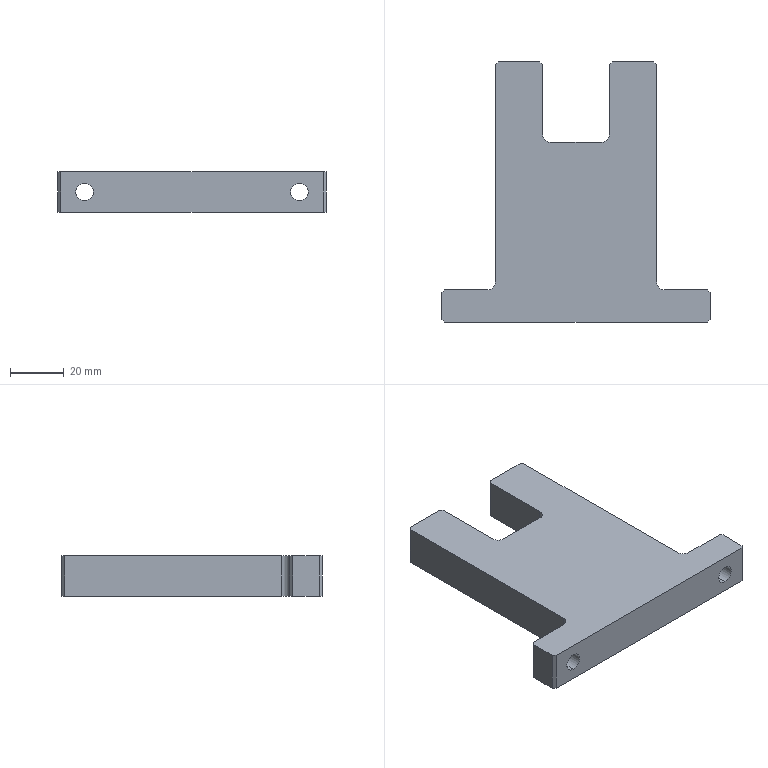Part | STEP file | 1 solid | 38 faces | box 100 x 97 x 15 mm | volume 82141 mm3 | plane 22 | cylinder 12 | cone 4 | commonest cylinder face diameters 4.2 x4 6 x4 6.6 x4